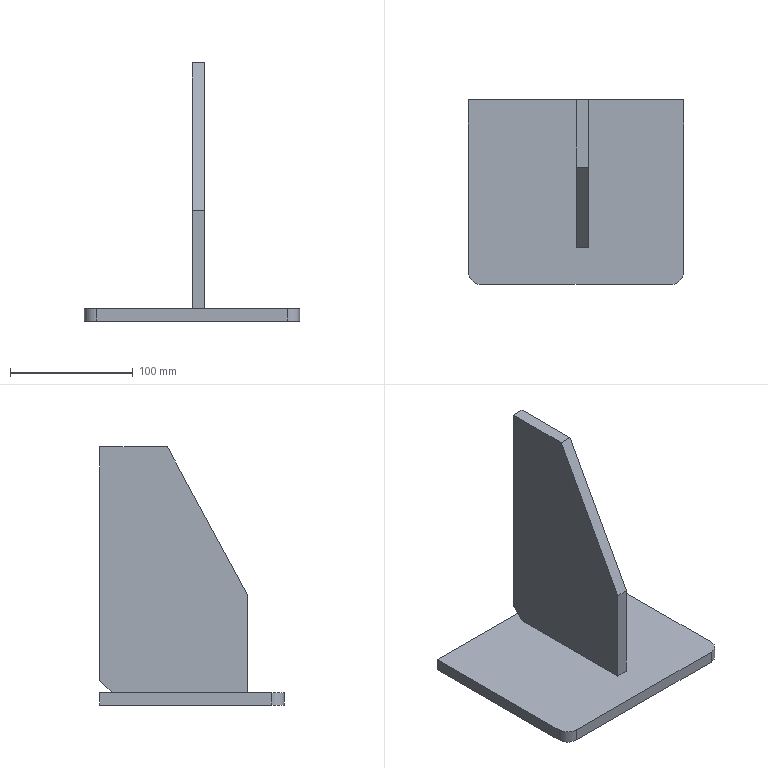Part | STEP file | PN_0029 web-top 10t steel corbel_Default<As Machined> | 2 solids | 16 faces | box 175 x 150 x 209.905 mm | volume 462571 mm3 | plane 13 | cylinder 2 | spline 1 | commonest cylinder face diameters 20 x2
STEP:
#1=CARTESIAN_POINT('',(0.,0.,0.));
#2=DIRECTION('',(0.,0.,1.));
#3=DIRECTION('',(1.,0.,0.));
#4=AXIS2_PLACEMENT_3D('',#1,#2,#3);
#5=CARTESIAN_POINT('',(77.5,-75.,0.));
#6=VERTEX_POINT('',#5);
#7=CARTESIAN_POINT('',(77.5,-75.,10.));
#8=VERTEX_POINT('',#7);
#9=CARTESIAN_POINT('',(77.5,-75.,10.));
#10=DIRECTION('',(0.,0.,1.));
#11=VECTOR('',#10,1.);
#12=LINE('',#9,#11);
#13=CARTESIAN_POINT('',(77.5,-65.,10.));
#14=DIRECTION('',(0.,0.,1.));
#15=DIRECTION('',(1.,0.,0.));
#16=AXIS2_PLACEMENT_3D('',#13,#14,#15);
#17=CYLINDRICAL_SURFACE('',#16,10.);
#18=CARTESIAN_POINT('',(4.712,0.));
#19=DIRECTION('',(0.,1.));
#20=VECTOR('',#19,1.);
#21=LINE('',#18,#20);
#22=(GEOMETRIC_REPRESENTATION_CONTEXT(2)PARAMETRIC_REPRESENTATION_CONTEXT()REPRESENTATION_CONTEXT('',''));
#23=DEFINITIONAL_REPRESENTATION('',(#21),#22);
#24=PCURVE('',#17,#23);
#25=CARTESIAN_POINT('',(-87.5,-75.,10.));
#26=DIRECTION('',(0.,1.,0.));
#27=DIRECTION('',(0.,0.,1.));
#28=AXIS2_PLACEMENT_3D('',#25,#26,#27);
#29=PLANE('',#28);
#30=CARTESIAN_POINT('',(0.,165.));
#31=DIRECTION('',(1.,0.));
#32=VECTOR('',#31,1.);
#33=LINE('',#30,#32);
#34=(GEOMETRIC_REPRESENTATION_CONTEXT(2)PARAMETRIC_REPRESENTATION_CONTEXT()REPRESENTATION_CONTEXT('',''));
#35=DEFINITIONAL_REPRESENTATION('',(#33),#34);
#36=PCURVE('',#29,#35);
#37=SURFACE_CURVE('',#12,(#24,#36),.PCURVE_S1.);
#38=EDGE_CURVE('',#6,#8,#37,.T.);
#39=ORIENTED_EDGE('',*,*,#38,.F.);
#40=CARTESIAN_POINT('',(87.5,-65.,0.));
#41=VERTEX_POINT('',#40);
#42=CARTESIAN_POINT('',(77.5,-65.,0.));
#43=DIRECTION('',(0.,0.,-1.));
#44=DIRECTION('',(1.,0.,0.));
#45=AXIS2_PLACEMENT_3D('',#42,#43,#44);
#46=CIRCLE('',#45,10.);
#47=CARTESIAN_POINT('',(6.283,-10.));
#48=DIRECTION('',(-1.,0.));
#49=VECTOR('',#48,1.);
#50=LINE('',#47,#49);
#51=(GEOMETRIC_REPRESENTATION_CONTEXT(2)PARAMETRIC_REPRESENTATION_CONTEXT()REPRESENTATION_CONTEXT('',''));
#52=DEFINITIONAL_REPRESENTATION('',(#50),#51);
#53=PCURVE('',#17,#52);
#54=CARTESIAN_POINT('',(0.,0.,0.));
#55=DIRECTION('',(0.,0.,1.));
#56=DIRECTION('',(1.,0.,0.));
#57=AXIS2_PLACEMENT_3D('',#54,#55,#56);
#58=PLANE('',#57);
#59=CARTESIAN_POINT('',(87.5,-65.));
#60=CARTESIAN_POINT('',(87.5,-82.321));
#61=CARTESIAN_POINT('',(72.5,-73.66));
#62=CARTESIAN_POINT('',(57.5,-65.));
#63=CARTESIAN_POINT('',(72.5,-56.34));
#64=CARTESIAN_POINT('',(87.5,-47.679));
#65=CARTESIAN_POINT('',(87.5,-65.));
#66=(BOUNDED_CURVE()B_SPLINE_CURVE(2,(#59,#60,#61,#62,#63,#64,#65),.UNSPECIFIED.,.T.,.F.)B_SPLINE_CURVE_WITH_KNOTS((1,2,2,2,2,1),(-2.094,0.,2.094,4.189,6.283,8.378),.UNSPECIFIED.)CURVE()GEOMETRIC_REPRESENTATION_ITEM()RATIONAL_B_SPLINE_CURVE((1.,0.5,1.,0.5,1.,0.5,1.))REPRESENTATION_ITEM(''));
#67=(GEOMETRIC_REPRESENTATION_CONTEXT(2)PARAMETRIC_REPRESENTATION_CONTEXT()REPRESENTATION_CONTEXT('',''));
#68=DEFINITIONAL_REPRESENTATION('',(#66),#67);
#69=PCURVE('',#58,#68);
#70=SURFACE_CURVE('',#46,(#53,#69),.PCURVE_S1.);
#71=EDGE_CURVE('',#41,#6,#70,.T.);
#72=ORIENTED_EDGE('',*,*,#71,.F.);
#73=CARTESIAN_POINT('',(87.5,-65.,10.));
#74=VERTEX_POINT('',#73);
#75=CARTESIAN_POINT('',(87.5,-65.,10.));
#76=DIRECTION('',(0.,0.,-1.));
#77=VECTOR('',#76,1.);
#78=LINE('',#75,#77);
#79=CARTESIAN_POINT('',(6.283,0.));
#80=DIRECTION('',(0.,-1.));
#81=VECTOR('',#80,1.);
#82=LINE('',#79,#81);
#83=(GEOMETRIC_REPRESENTATION_CONTEXT(2)PARAMETRIC_REPRESENTATION_CONTEXT()REPRESENTATION_CONTEXT('',''));
#84=DEFINITIONAL_REPRESENTATION('',(#82),#83);
#85=PCURVE('',#17,#84);
#86=CARTESIAN_POINT('',(87.5,75.,10.));
#87=DIRECTION('',(-1.,0.,0.));
#88=DIRECTION('',(0.,0.,1.));
#89=AXIS2_PLACEMENT_3D('',#86,#87,#88);
#90=PLANE('',#89);
#91=CARTESIAN_POINT('',(0.,-140.));
#92=DIRECTION('',(-1.,0.));
#93=VECTOR('',#92,1.);
#94=LINE('',#91,#93);
#95=(GEOMETRIC_REPRESENTATION_CONTEXT(2)PARAMETRIC_REPRESENTATION_CONTEXT()REPRESENTATION_CONTEXT('',''));
#96=DEFINITIONAL_REPRESENTATION('',(#94),#95);
#97=PCURVE('',#90,#96);
#98=SURFACE_CURVE('',#78,(#85,#97),.PCURVE_S1.);
#99=EDGE_CURVE('',#74,#41,#98,.T.);
#100=ORIENTED_EDGE('',*,*,#99,.F.);
#101=CARTESIAN_POINT('',(77.5,-65.,10.));
#102=DIRECTION('',(0.,0.,1.));
#103=DIRECTION('',(1.,0.,0.));
#104=AXIS2_PLACEMENT_3D('',#101,#102,#103);
#105=CIRCLE('',#104,10.);
#106=CARTESIAN_POINT('',(0.,0.));
#107=DIRECTION('',(1.,0.));
#108=VECTOR('',#107,1.);
#109=LINE('',#106,#108);
#110=(GEOMETRIC_REPRESENTATION_CONTEXT(2)PARAMETRIC_REPRESENTATION_CONTEXT()REPRESENTATION_CONTEXT('',''));
#111=DEFINITIONAL_REPRESENTATION('',(#109),#110);
#112=PCURVE('',#17,#111);
#113=CARTESIAN_POINT('',(0.,0.,10.));
#114=DIRECTION('',(0.,0.,1.));
#115=DIRECTION('',(1.,0.,0.));
#116=AXIS2_PLACEMENT_3D('',#113,#114,#115);
#117=PLANE('',#116);
#118=CARTESIAN_POINT('',(77.5,-65.));
#119=DIRECTION('',(1.,0.));
#120=AXIS2_PLACEMENT_2D('',#118,#119);
#121=CIRCLE('',#120,10.);
#122=(GEOMETRIC_REPRESENTATION_CONTEXT(2)PARAMETRIC_REPRESENTATION_CONTEXT()REPRESENTATION_CONTEXT('',''));
#123=DEFINITIONAL_REPRESENTATION('',(#121),#122);
#124=PCURVE('',#117,#123);
#125=SURFACE_CURVE('',#105,(#112,#124),.PCURVE_S1.);
#126=EDGE_CURVE('',#8,#74,#125,.T.);
#127=ORIENTED_EDGE('',*,*,#126,.F.);
#128=EDGE_LOOP('',(#39,#72,#100,#127));
#129=FACE_BOUND('',#128,.T.);
#130=ADVANCED_FACE('',(#129),#17,.T.);
#131=CARTESIAN_POINT('',(-87.5,-65.,0.));
#132=VERTEX_POINT('',#131);
#133=CARTESIAN_POINT('',(-87.5,-65.,10.));
#134=VERTEX_POINT('',#133);
#135=CARTESIAN_POINT('',(-87.5,-65.,10.));
#136=DIRECTION('',(0.,0.,1.));
#137=VECTOR('',#136,1.);
#138=LINE('',#135,#137);
#139=CARTESIAN_POINT('',(-77.5,-65.,10.));
#140=DIRECTION('',(0.,0.,1.));
#141=DIRECTION('',(1.,0.,0.));
#142=AXIS2_PLACEMENT_3D('',#139,#140,#141);
#143=CYLINDRICAL_SURFACE('',#142,10.);
#144=CARTESIAN_POINT('',(3.142,0.));
#145=DIRECTION('',(0.,1.));
#146=VECTOR('',#145,1.);
#147=LINE('',#144,#146);
#148=(GEOMETRIC_REPRESENTATION_CONTEXT(2)PARAMETRIC_REPRESENTATION_CONTEXT()REPRESENTATION_CONTEXT('',''));
#149=DEFINITIONAL_REPRESENTATION('',(#147),#148);
#150=PCURVE('',#143,#149);
#151=CARTESIAN_POINT('',(-87.5,75.,10.));
#152=DIRECTION('',(1.,0.,0.));
#153=DIRECTION('',(0.,0.,-1.));
#154=AXIS2_PLACEMENT_3D('',#151,#152,#153);
#155=PLANE('',#154);
#156=CARTESIAN_POINT('',(0.,-140.));
#157=DIRECTION('',(-1.,0.));
#158=VECTOR('',#157,1.);
#159=LINE('',#156,#158);
#160=(GEOMETRIC_REPRESENTATION_CONTEXT(2)PARAMETRIC_REPRESENTATION_CONTEXT()REPRESENTATION_CONTEXT('',''));
#161=DEFINITIONAL_REPRESENTATION('',(#159),#160);
#162=PCURVE('',#155,#161);
#163=SURFACE_CURVE('',#138,(#150,#162),.PCURVE_S1.);
#164=EDGE_CURVE('',#132,#134,#163,.T.);
#165=ORIENTED_EDGE('',*,*,#164,.F.);
#166=CARTESIAN_POINT('',(-77.5,-75.,0.));
#167=VERTEX_POINT('',#166);
#168=CARTESIAN_POINT('',(-77.5,-65.,0.));
#169=DIRECTION('',(0.,0.,-1.));
#170=DIRECTION('',(1.,0.,0.));
#171=AXIS2_PLACEMENT_3D('',#168,#169,#170);
#172=CIRCLE('',#171,10.);
#173=CARTESIAN_POINT('',(6.283,-10.));
#174=DIRECTION('',(-1.,0.));
#175=VECTOR('',#174,1.);
#176=LINE('',#173,#175);
#177=(GEOMETRIC_REPRESENTATION_CONTEXT(2)PARAMETRIC_REPRESENTATION_CONTEXT()REPRESENTATION_CONTEXT('',''));
#178=DEFINITIONAL_REPRESENTATION('',(#176),#177);
#179=PCURVE('',#143,#178);
#180=CARTESIAN_POINT('',(-67.5,-65.));
#181=CARTESIAN_POINT('',(-67.5,-82.321));
#182=CARTESIAN_POINT('',(-82.5,-73.66));
#183=CARTESIAN_POINT('',(-97.5,-65.));
#184=CARTESIAN_POINT('',(-82.5,-56.34));
#185=CARTESIAN_POINT('',(-67.5,-47.679));
#186=CARTESIAN_POINT('',(-67.5,-65.));
#187=(BOUNDED_CURVE()B_SPLINE_CURVE(2,(#180,#181,#182,#183,#184,#185,#186),.UNSPECIFIED.,.T.,.F.)B_SPLINE_CURVE_WITH_KNOTS((1,2,2,2,2,1),(-2.094,0.,2.094,4.189,6.283,8.378),.UNSPECIFIED.)CURVE()GEOMETRIC_REPRESENTATION_ITEM()RATIONAL_B_SPLINE_CURVE((1.,0.5,1.,0.5,1.,0.5,1.))REPRESENTATION_ITEM(''));
#188=(GEOMETRIC_REPRESENTATION_CONTEXT(2)PARAMETRIC_REPRESENTATION_CONTEXT()REPRESENTATION_CONTEXT('',''));
#189=DEFINITIONAL_REPRESENTATION('',(#187),#188);
#190=PCURVE('',#58,#189);
#191=SURFACE_CURVE('',#172,(#179,#190),.PCURVE_S1.);
#192=EDGE_CURVE('',#167,#132,#191,.T.);
#193=ORIENTED_EDGE('',*,*,#192,.F.);
#194=CARTESIAN_POINT('',(-77.5,-75.,10.));
#195=VERTEX_POINT('',#194);
#196=CARTESIAN_POINT('',(-77.5,-75.,10.));
#197=DIRECTION('',(0.,0.,-1.));
#198=VECTOR('',#197,1.);
#199=LINE('',#196,#198);
#200=CARTESIAN_POINT('',(4.712,0.));
#201=DIRECTION('',(0.,-1.));
#202=VECTOR('',#201,1.);
#203=LINE('',#200,#202);
#204=(GEOMETRIC_REPRESENTATION_CONTEXT(2)PARAMETRIC_REPRESENTATION_CONTEXT()REPRESENTATION_CONTEXT('',''));
#205=DEFINITIONAL_REPRESENTATION('',(#203),#204);
#206=PCURVE('',#143,#205);
#207=CARTESIAN_POINT('',(0.,10.));
#208=DIRECTION('',(-1.,0.));
#209=VECTOR('',#208,1.);
#210=LINE('',#207,#209);
#211=(GEOMETRIC_REPRESENTATION_CONTEXT(2)PARAMETRIC_REPRESENTATION_CONTEXT()REPRESENTATION_CONTEXT('',''));
#212=DEFINITIONAL_REPRESENTATION('',(#210),#211);
#213=PCURVE('',#29,#212);
#214=SURFACE_CURVE('',#199,(#206,#213),.PCURVE_S1.);
#215=EDGE_CURVE('',#195,#167,#214,.T.);
#216=ORIENTED_EDGE('',*,*,#215,.F.);
#217=CARTESIAN_POINT('',(-77.5,-65.,10.));
#218=DIRECTION('',(0.,0.,1.));
#219=DIRECTION('',(1.,0.,0.));
#220=AXIS2_PLACEMENT_3D('',#217,#218,#219);
#221=CIRCLE('',#220,10.);
#222=CARTESIAN_POINT('',(0.,0.));
#223=DIRECTION('',(1.,0.));
#224=VECTOR('',#223,1.);
#225=LINE('',#222,#224);
#226=(GEOMETRIC_REPRESENTATION_CONTEXT(2)PARAMETRIC_REPRESENTATION_CONTEXT()REPRESENTATION_CONTEXT('',''));
#227=DEFINITIONAL_REPRESENTATION('',(#225),#226);
#228=PCURVE('',#143,#227);
#229=CARTESIAN_POINT('',(-77.5,-65.));
#230=DIRECTION('',(1.,0.));
#231=AXIS2_PLACEMENT_2D('',#229,#230);
#232=CIRCLE('',#231,10.);
#233=(GEOMETRIC_REPRESENTATION_CONTEXT(2)PARAMETRIC_REPRESENTATION_CONTEXT()REPRESENTATION_CONTEXT('',''));
#234=DEFINITIONAL_REPRESENTATION('',(#232),#233);
#235=PCURVE('',#117,#234);
#236=SURFACE_CURVE('',#221,(#228,#235),.PCURVE_S1.);
#237=EDGE_CURVE('',#134,#195,#236,.T.);
#238=ORIENTED_EDGE('',*,*,#237,.F.);
#239=EDGE_LOOP('',(#165,#193,#216,#238));
#240=FACE_BOUND('',#239,.T.);
#241=ADVANCED_FACE('',(#240),#143,.T.);
#242=CARTESIAN_POINT('',(87.5,75.,10.));
#243=VERTEX_POINT('',#242);
#244=CARTESIAN_POINT('',(87.5,75.,10.));
#245=DIRECTION('',(0.,1.,0.));
#246=VECTOR('',#245,1.);
#247=LINE('',#244,#246);
#248=CARTESIAN_POINT('',(0.,0.));
#249=DIRECTION('',(0.,1.));
#250=VECTOR('',#249,1.);
#251=LINE('',#248,#250);
#252=(GEOMETRIC_REPRESENTATION_CONTEXT(2)PARAMETRIC_REPRESENTATION_CONTEXT()REPRESENTATION_CONTEXT('',''));
#253=DEFINITIONAL_REPRESENTATION('',(#251),#252);
#254=PCURVE('',#90,#253);
#255=CARTESIAN_POINT('',(87.5,75.));
#256=DIRECTION('',(0.,1.));
#257=VECTOR('',#256,1.);
#258=LINE('',#255,#257);
#259=(GEOMETRIC_REPRESENTATION_CONTEXT(2)PARAMETRIC_REPRESENTATION_CONTEXT()REPRESENTATION_CONTEXT('',''));
#260=DEFINITIONAL_REPRESENTATION('',(#258),#259);
#261=PCURVE('',#117,#260);
#262=SURFACE_CURVE('',#247,(#254,#261),.PCURVE_S1.);
#263=EDGE_CURVE('',#74,#243,#262,.T.);
#264=ORIENTED_EDGE('',*,*,#263,.F.);
#265=ORIENTED_EDGE('',*,*,#99,.T.);
#266=CARTESIAN_POINT('',(87.5,75.,0.));
#267=VERTEX_POINT('',#266);
#268=CARTESIAN_POINT('',(87.5,75.,0.));
#269=DIRECTION('',(0.,1.,0.));
#270=VECTOR('',#269,1.);
#271=LINE('',#268,#270);
#272=CARTESIAN_POINT('',(-10.,0.));
#273=DIRECTION('',(0.,1.));
#274=VECTOR('',#273,1.);
#275=LINE('',#272,#274);
#276=(GEOMETRIC_REPRESENTATION_CONTEXT(2)PARAMETRIC_REPRESENTATION_CONTEXT()REPRESENTATION_CONTEXT('',''));
#277=DEFINITIONAL_REPRESENTATION('',(#275),#276);
#278=PCURVE('',#90,#277);
#279=CARTESIAN_POINT('',(87.5,75.));
#280=DIRECTION('',(0.,1.));
#281=VECTOR('',#280,1.);
#282=LINE('',#279,#281);
#283=(GEOMETRIC_REPRESENTATION_CONTEXT(2)PARAMETRIC_REPRESENTATION_CONTEXT()REPRESENTATION_CONTEXT('',''));
#284=DEFINITIONAL_REPRESENTATION('',(#282),#283);
#285=PCURVE('',#58,#284);
#286=SURFACE_CURVE('',#271,(#278,#285),.PCURVE_S1.);
#287=EDGE_CURVE('',#41,#267,#286,.T.);
#288=ORIENTED_EDGE('',*,*,#287,.T.);
#289=CARTESIAN_POINT('',(87.5,75.,10.));
#290=DIRECTION('',(0.,0.,-1.));
#291=VECTOR('',#290,1.);
#292=LINE('',#289,#291);
#293=CARTESIAN_POINT('',(0.,0.));
#294=DIRECTION('',(-1.,0.));
#295=VECTOR('',#294,1.);
#296=LINE('',#293,#295);
#297=(GEOMETRIC_REPRESENTATION_CONTEXT(2)PARAMETRIC_REPRESENTATION_CONTEXT()REPRESENTATION_CONTEXT('',''));
#298=DEFINITIONAL_REPRESENTATION('',(#296),#297);
#299=PCURVE('',#90,#298);
#300=CARTESIAN_POINT('',(-87.5,75.,10.));
#301=DIRECTION('',(0.,-1.,0.));
#302=DIRECTION('',(0.,0.,-1.));
#303=AXIS2_PLACEMENT_3D('',#300,#301,#302);
#304=PLANE('',#303);
#305=CARTESIAN_POINT('',(0.,175.));
#306=DIRECTION('',(1.,0.));
#307=VECTOR('',#306,1.);
#308=LINE('',#305,#307);
#309=(GEOMETRIC_REPRESENTATION_CONTEXT(2)PARAMETRIC_REPRESENTATION_CONTEXT()REPRESENTATION_CONTEXT('',''));
#310=DEFINITIONAL_REPRESENTATION('',(#308),#309);
#311=PCURVE('',#304,#310);
#312=SURFACE_CURVE('',#292,(#299,#311),.PCURVE_S1.);
#313=EDGE_CURVE('',#243,#267,#312,.T.);
#314=ORIENTED_EDGE('',*,*,#313,.F.);
#315=EDGE_LOOP('',(#264,#265,#288,#314));
#316=FACE_BOUND('',#315,.T.);
#317=ADVANCED_FACE('',(#316),#90,.F.);
#318=CARTESIAN_POINT('',(-87.5,75.,0.));
#319=VERTEX_POINT('',#318);
#320=CARTESIAN_POINT('',(-87.5,75.,0.));
#321=DIRECTION('',(-1.,0.,0.));
#322=VECTOR('',#321,1.);
#323=LINE('',#320,#322);
#324=CARTESIAN_POINT('',(10.,0.));
#325=DIRECTION('',(0.,-1.));
#326=VECTOR('',#325,1.);
#327=LINE('',#324,#326);
#328=(GEOMETRIC_REPRESENTATION_CONTEXT(2)PARAMETRIC_REPRESENTATION_CONTEXT()REPRESENTATION_CONTEXT('',''));
#329=DEFINITIONAL_REPRESENTATION('',(#327),#328);
#330=PCURVE('',#304,#329);
#331=CARTESIAN_POINT('',(-87.5,75.));
#332=DIRECTION('',(-1.,0.));
#333=VECTOR('',#332,1.);
#334=LINE('',#331,#333);
#335=(GEOMETRIC_REPRESENTATION_CONTEXT(2)PARAMETRIC_REPRESENTATION_CONTEXT()REPRESENTATION_CONTEXT('',''));
#336=DEFINITIONAL_REPRESENTATION('',(#334),#335);
#337=PCURVE('',#58,#336);
#338=SURFACE_CURVE('',#323,(#330,#337),.PCURVE_S1.);
#339=EDGE_CURVE('',#267,#319,#338,.T.);
#340=ORIENTED_EDGE('',*,*,#339,.T.);
#341=CARTESIAN_POINT('',(-87.5,75.,10.));
#342=VERTEX_POINT('',#341);
#343=CARTESIAN_POINT('',(-87.5,75.,10.));
#344=DIRECTION('',(0.,0.,-1.));
#345=VECTOR('',#344,1.);
#346=LINE('',#343,#345);
#347=CARTESIAN_POINT('',(0.,0.));
#348=DIRECTION('',(1.,0.));
#349=VECTOR('',#348,1.);
#350=LINE('',#347,#349);
#351=(GEOMETRIC_REPRESENTATION_CONTEXT(2)PARAMETRIC_REPRESENTATION_CONTEXT()REPRESENTATION_CONTEXT('',''));
#352=DEFINITIONAL_REPRESENTATION('',(#350),#351);
#353=PCURVE('',#304,#352);
#354=CARTESIAN_POINT('',(0.,0.));
#355=DIRECTION('',(1.,0.));
#356=VECTOR('',#355,1.);
#357=LINE('',#354,#356);
#358=(GEOMETRIC_REPRESENTATION_CONTEXT(2)PARAMETRIC_REPRESENTATION_CONTEXT()REPRESENTATION_CONTEXT('',''));
#359=DEFINITIONAL_REPRESENTATION('',(#357),#358);
#360=PCURVE('',#155,#359);
#361=SURFACE_CURVE('',#346,(#353,#360),.PCURVE_S1.);
#362=EDGE_CURVE('',#342,#319,#361,.T.);
#363=ORIENTED_EDGE('',*,*,#362,.F.);
#364=CARTESIAN_POINT('',(-87.5,75.,10.));
#365=DIRECTION('',(-1.,0.,0.));
#366=VECTOR('',#365,1.);
#367=LINE('',#364,#366);
#368=CARTESIAN_POINT('',(0.,0.));
#369=DIRECTION('',(0.,-1.));
#370=VECTOR('',#369,1.);
#371=LINE('',#368,#370);
#372=(GEOMETRIC_REPRESENTATION_CONTEXT(2)PARAMETRIC_REPRESENTATION_CONTEXT()REPRESENTATION_CONTEXT('',''));
#373=DEFINITIONAL_REPRESENTATION('',(#371),#372);
#374=PCURVE('',#304,#373);
#375=CARTESIAN_POINT('',(-87.5,75.));
#376=DIRECTION('',(-1.,0.));
#377=VECTOR('',#376,1.);
#378=LINE('',#375,#377);
#379=(GEOMETRIC_REPRESENTATION_CONTEXT(2)PARAMETRIC_REPRESENTATION_CONTEXT()REPRESENTATION_CONTEXT('',''));
#380=DEFINITIONAL_REPRESENTATION('',(#378),#379);
#381=PCURVE('',#117,#380);
#382=SURFACE_CURVE('',#367,(#374,#381),.PCURVE_S1.);
#383=EDGE_CURVE('',#243,#342,#382,.T.);
#384=ORIENTED_EDGE('',*,*,#383,.F.);
#385=ORIENTED_EDGE('',*,*,#313,.T.);
#386=EDGE_LOOP('',(#340,#363,#384,#385));
#387=FACE_BOUND('',#386,.T.);
#388=ADVANCED_FACE('',(#387),#304,.F.);
#389=CARTESIAN_POINT('',(-87.5,75.,0.));
#390=DIRECTION('',(0.,-1.,0.));
#391=VECTOR('',#390,1.);
#392=LINE('',#389,#391);
#393=CARTESIAN_POINT('',(10.,0.));
#394=DIRECTION('',(0.,-1.));
#395=VECTOR('',#394,1.);
#396=LINE('',#393,#395);
#397=(GEOMETRIC_REPRESENTATION_CONTEXT(2)PARAMETRIC_REPRESENTATION_CONTEXT()REPRESENTATION_CONTEXT('',''));
#398=DEFINITIONAL_REPRESENTATION('',(#396),#397);
#399=PCURVE('',#155,#398);
#400=CARTESIAN_POINT('',(-87.5,75.));
#401=DIRECTION('',(0.,-1.));
#402=VECTOR('',#401,1.);
#403=LINE('',#400,#402);
#404=(GEOMETRIC_REPRESENTATION_CONTEXT(2)PARAMETRIC_REPRESENTATION_CONTEXT()REPRESENTATION_CONTEXT('',''));
#405=DEFINITIONAL_REPRESENTATION('',(#403),#404);
#406=PCURVE('',#58,#405);
#407=SURFACE_CURVE('',#392,(#399,#406),.PCURVE_S1.);
#408=EDGE_CURVE('',#319,#132,#407,.T.);
#409=ORIENTED_EDGE('',*,*,#408,.T.);
#410=ORIENTED_EDGE('',*,*,#164,.T.);
#411=CARTESIAN_POINT('',(-87.5,75.,10.));
#412=DIRECTION('',(0.,-1.,0.));
#413=VECTOR('',#412,1.);
#414=LINE('',#411,#413);
#415=CARTESIAN_POINT('',(0.,0.));
#416=DIRECTION('',(0.,-1.));
#417=VECTOR('',#416,1.);
#418=LINE('',#415,#417);
#419=(GEOMETRIC_REPRESENTATION_CONTEXT(2)PARAMETRIC_REPRESENTATION_CONTEXT()REPRESENTATION_CONTEXT('',''));
#420=DEFINITIONAL_REPRESENTATION('',(#418),#419);
#421=PCURVE('',#155,#420);
#422=CARTESIAN_POINT('',(-87.5,75.));
#423=DIRECTION('',(0.,-1.));
#424=VECTOR('',#423,1.);
#425=LINE('',#422,#424);
#426=(GEOMETRIC_REPRESENTATION_CONTEXT(2)PARAMETRIC_REPRESENTATION_CONTEXT()REPRESENTATION_CONTEXT('',''));
#427=DEFINITIONAL_REPRESENTATION('',(#425),#426);
#428=PCURVE('',#117,#427);
#429=SURFACE_CURVE('',#414,(#421,#428),.PCURVE_S1.);
#430=EDGE_CURVE('',#342,#134,#429,.T.);
#431=ORIENTED_EDGE('',*,*,#430,.F.);
#432=ORIENTED_EDGE('',*,*,#362,.T.);
#433=EDGE_LOOP('',(#409,#410,#431,#432));
#434=FACE_BOUND('',#433,.T.);
#435=ADVANCED_FACE('',(#434),#155,.F.);
#436=CARTESIAN_POINT('',(-87.5,-75.,0.));
#437=DIRECTION('',(1.,0.,0.));
#438=VECTOR('',#437,1.);
#439=LINE('',#436,#438);
#440=CARTESIAN_POINT('',(-10.,0.));
#441=DIRECTION('',(0.,1.));
#442=VECTOR('',#441,1.);
#443=LINE('',#440,#442);
#444=(GEOMETRIC_REPRESENTATION_CONTEXT(2)PARAMETRIC_REPRESENTATION_CONTEXT()REPRESENTATION_CONTEXT('',''));
#445=DEFINITIONAL_REPRESENTATION('',(#443),#444);
#446=PCURVE('',#29,#445);
#447=CARTESIAN_POINT('',(-87.5,-75.));
#448=DIRECTION('',(1.,0.));
#449=VECTOR('',#448,1.);
#450=LINE('',#447,#449);
#451=(GEOMETRIC_REPRESENTATION_CONTEXT(2)PARAMETRIC_REPRESENTATION_CONTEXT()REPRESENTATION_CONTEXT('',''));
#452=DEFINITIONAL_REPRESENTATION('',(#450),#451);
#453=PCURVE('',#58,#452);
#454=SURFACE_CURVE('',#439,(#446,#453),.PCURVE_S1.);
#455=EDGE_CURVE('',#167,#6,#454,.T.);
#456=ORIENTED_EDGE('',*,*,#455,.T.);
#457=ORIENTED_EDGE('',*,*,#38,.T.);
#458=CARTESIAN_POINT('',(-87.5,-75.,10.));
#459=DIRECTION('',(1.,0.,0.));
#460=VECTOR('',#459,1.);
#461=LINE('',#458,#460);
#462=CARTESIAN_POINT('',(0.,0.));
#463=DIRECTION('',(0.,1.));
#464=VECTOR('',#463,1.);
#465=LINE('',#462,#464);
#466=(GEOMETRIC_REPRESENTATION_CONTEXT(2)PARAMETRIC_REPRESENTATION_CONTEXT()REPRESENTATION_CONTEXT('',''));
#467=DEFINITIONAL_REPRESENTATION('',(#465),#466);
#468=PCURVE('',#29,#467);
#469=CARTESIAN_POINT('',(-87.5,-75.));
#470=DIRECTION('',(1.,0.));
#471=VECTOR('',#470,1.);
#472=LINE('',#469,#471);
#473=(GEOMETRIC_REPRESENTATION_CONTEXT(2)PARAMETRIC_REPRESENTATION_CONTEXT()REPRESENTATION_CONTEXT('',''));
#474=DEFINITIONAL_REPRESENTATION('',(#472),#473);
#475=PCURVE('',#117,#474);
#476=SURFACE_CURVE('',#461,(#468,#475),.PCURVE_S1.);
#477=EDGE_CURVE('',#195,#8,#476,.T.);
#478=ORIENTED_EDGE('',*,*,#477,.F.);
#479=ORIENTED_EDGE('',*,*,#215,.T.);
#480=EDGE_LOOP('',(#456,#457,#478,#479));
#481=FACE_BOUND('',#480,.T.);
#482=ADVANCED_FACE('',(#481),#29,.F.);
#483=ORIENTED_EDGE('',*,*,#477,.T.);
#484=ORIENTED_EDGE('',*,*,#126,.T.);
#485=ORIENTED_EDGE('',*,*,#263,.T.);
#486=ORIENTED_EDGE('',*,*,#383,.T.);
#487=ORIENTED_EDGE('',*,*,#430,.T.);
#488=ORIENTED_EDGE('',*,*,#237,.T.);
#489=EDGE_LOOP('',(#483,#484,#485,#486,#487,#488));
#490=FACE_BOUND('',#489,.T.);
#491=ADVANCED_FACE('',(#490),#117,.T.);
#492=ORIENTED_EDGE('',*,*,#287,.F.);
#493=ORIENTED_EDGE('',*,*,#71,.T.);
#494=ORIENTED_EDGE('',*,*,#455,.F.);
#495=ORIENTED_EDGE('',*,*,#192,.T.);
#496=ORIENTED_EDGE('',*,*,#408,.F.);
#497=ORIENTED_EDGE('',*,*,#339,.F.);
#498=EDGE_LOOP('',(#492,#493,#494,#495,#496,#497));
#499=FACE_BOUND('',#498,.T.);
#500=ADVANCED_FACE('',(#499),#58,.F.);
#501=CLOSED_SHELL('',(#130,#241,#317,#388,#435,#482,#491,#500));
#502=MANIFOLD_SOLID_BREP('',#501);
#503=CARTESIAN_POINT('',(0.,64.998,9.905));
#504=VERTEX_POINT('',#503);
#505=CARTESIAN_POINT('',(10.,64.998,9.905));
#506=VERTEX_POINT('',#505);
#507=CARTESIAN_POINT('',(10.,64.998,9.905));
#508=DIRECTION('',(1.,0.,0.));
#509=VECTOR('',#508,1.);
#510=LINE('',#507,#509);
#511=CARTESIAN_POINT('',(10.,64.998,9.905));
#512=DIRECTION('',(0.,-0.7071,0.7071));
#513=DIRECTION('',(1.,0.,0.));
#514=AXIS2_PLACEMENT_3D('',#511,#512,#513);
#515=PLANE('',#514);
#516=CARTESIAN_POINT('',(0.,0.));
#517=DIRECTION('',(1.,0.));
#518=VECTOR('',#517,1.);
#519=LINE('',#516,#518);
#520=(GEOMETRIC_REPRESENTATION_CONTEXT(2)PARAMETRIC_REPRESENTATION_CONTEXT()REPRESENTATION_CONTEXT('',''));
#521=DEFINITIONAL_REPRESENTATION('',(#519),#520);
#522=PCURVE('',#515,#521);
#523=CARTESIAN_POINT('',(10.,74.998,9.905));
#524=DIRECTION('',(0.,0.,1.));
#525=DIRECTION('',(1.,0.,0.));
#526=AXIS2_PLACEMENT_3D('',#523,#524,#525);
#527=PLANE('',#526);
#528=CARTESIAN_POINT('',(0.,-10.));
#529=DIRECTION('',(1.,0.));
#530=VECTOR('',#529,1.);
#531=LINE('',#528,#530);
#532=(GEOMETRIC_REPRESENTATION_CONTEXT(2)PARAMETRIC_REPRESENTATION_CONTEXT()REPRESENTATION_CONTEXT('',''));
#533=DEFINITIONAL_REPRESENTATION('',(#531),#532);
#534=PCURVE('',#527,#533);
#535=SURFACE_CURVE('',#510,(#522,#534),.PCURVE_S1.);
#536=EDGE_CURVE('',#504,#506,#535,.T.);
#537=ORIENTED_EDGE('',*,*,#536,.F.);
#538=CARTESIAN_POINT('',(0.,74.998,19.905));
#539=VERTEX_POINT('',#538);
#540=CARTESIAN_POINT('',(0.,-1.144,-56.236));
#541=DIRECTION('',(0.,-0.7071,-0.7071));
#542=VECTOR('',#541,1.);
#543=LINE('',#540,#542);
#544=CARTESIAN_POINT('',(-10.,-93.538));
#545=DIRECTION('',(0.,-1.));
#546=VECTOR('',#545,1.);
#547=LINE('',#544,#546);
#548=(GEOMETRIC_REPRESENTATION_CONTEXT(2)PARAMETRIC_REPRESENTATION_CONTEXT()REPRESENTATION_CONTEXT('',''));
#549=DEFINITIONAL_REPRESENTATION('',(#547),#548);
#550=PCURVE('',#515,#549);
#551=CARTESIAN_POINT('',(0.,-37.84,-19.54));
#552=DIRECTION('',(-1.,0.,0.));
#553=DIRECTION('',(0.,0.,1.));
#554=AXIS2_PLACEMENT_3D('',#551,#552,#553);
#555=PLANE('',#554);
#556=CARTESIAN_POINT('',(-36.696,36.696));
#557=DIRECTION('',(-0.7071,-0.7071));
#558=VECTOR('',#557,1.);
#559=LINE('',#556,#558);
#560=(GEOMETRIC_REPRESENTATION_CONTEXT(2)PARAMETRIC_REPRESENTATION_CONTEXT()REPRESENTATION_CONTEXT('',''));
#561=DEFINITIONAL_REPRESENTATION('',(#559),#560);
#562=PCURVE('',#555,#561);
#563=SURFACE_CURVE('',#543,(#550,#562),.PCURVE_S1.);
#564=EDGE_CURVE('',#539,#504,#563,.T.);
#565=ORIENTED_EDGE('',*,*,#564,.F.);
#566=CARTESIAN_POINT('',(10.,74.998,19.905));
#567=VERTEX_POINT('',#566);
#568=CARTESIAN_POINT('',(10.,74.998,19.905));
#569=DIRECTION('',(-1.,0.,0.));
#570=VECTOR('',#569,1.);
#571=LINE('',#568,#570);
#572=CARTESIAN_POINT('',(0.,14.142));
#573=DIRECTION('',(-1.,0.));
#574=VECTOR('',#573,1.);
#575=LINE('',#572,#574);
#576=(GEOMETRIC_REPRESENTATION_CONTEXT(2)PARAMETRIC_REPRESENTATION_CONTEXT()REPRESENTATION_CONTEXT('',''));
#577=DEFINITIONAL_REPRESENTATION('',(#575),#576);
#578=PCURVE('',#515,#577);
#579=CARTESIAN_POINT('',(10.,74.998,9.905));
#580=DIRECTION('',(0.,-1.,0.));
#581=DIRECTION('',(0.,0.,-1.));
#582=AXIS2_PLACEMENT_3D('',#579,#580,#581);
#583=PLANE('',#582);
#584=CARTESIAN_POINT('',(-10.,0.));
#585=DIRECTION('',(0.,-1.));
#586=VECTOR('',#585,1.);
#587=LINE('',#584,#586);
#588=(GEOMETRIC_REPRESENTATION_CONTEXT(2)PARAMETRIC_REPRESENTATION_CONTEXT()REPRESENTATION_CONTEXT('',''));
#589=DEFINITIONAL_REPRESENTATION('',(#587),#588);
#590=PCURVE('',#583,#589);
#591=SURFACE_CURVE('',#571,(#578,#590),.PCURVE_S1.);
#592=EDGE_CURVE('',#567,#539,#591,.T.);
#593=ORIENTED_EDGE('',*,*,#592,.F.);
#594=CARTESIAN_POINT('',(10.,64.998,9.905));
#595=DIRECTION('',(0.,0.7071,0.7071));
#596=VECTOR('',#595,1.);
#597=LINE('',#594,#596);
#598=CARTESIAN_POINT('',(0.,0.));
#599=DIRECTION('',(0.,1.));
#600=VECTOR('',#599,1.);
#601=LINE('',#598,#600);
#602=(GEOMETRIC_REPRESENTATION_CONTEXT(2)PARAMETRIC_REPRESENTATION_CONTEXT()REPRESENTATION_CONTEXT('',''));
#603=DEFINITIONAL_REPRESENTATION('',(#601),#602);
#604=PCURVE('',#515,#603);
#605=CARTESIAN_POINT('',(10.,-37.84,-19.54));
#606=DIRECTION('',(-1.,0.,0.));
#607=DIRECTION('',(0.,0.,1.));
#608=AXIS2_PLACEMENT_3D('',#605,#606,#607);
#609=PLANE('',#608);
#610=CARTESIAN_POINT('',(29.445,102.838));
#611=DIRECTION('',(0.7071,0.7071));
#612=VECTOR('',#611,1.);
#613=LINE('',#610,#612);
#614=(GEOMETRIC_REPRESENTATION_CONTEXT(2)PARAMETRIC_REPRESENTATION_CONTEXT()REPRESENTATION_CONTEXT('',''));
#615=DEFINITIONAL_REPRESENTATION('',(#613),#614);
#616=PCURVE('',#609,#615);
#617=SURFACE_CURVE('',#597,(#604,#616),.PCURVE_S1.);
#618=EDGE_CURVE('',#506,#567,#617,.T.);
#619=ORIENTED_EDGE('',*,*,#618,.F.);
#620=EDGE_LOOP('',(#537,#565,#593,#619));
#621=FACE_BOUND('',#620,.T.);
#622=ADVANCED_FACE('',(#621),#515,.F.);
#623=CARTESIAN_POINT('',(0.,19.998,209.905));
#624=VERTEX_POINT('',#623);
#625=CARTESIAN_POINT('',(10.,19.998,209.905));
#626=VERTEX_POINT('',#625);
#627=CARTESIAN_POINT('',(0.,19.998,209.905));
#628=CARTESIAN_POINT('',(3.333,19.998,209.905));
#629=CARTESIAN_POINT('',(6.667,19.998,209.905));
#630=CARTESIAN_POINT('',(10.,19.998,209.905));
#631=B_SPLINE_CURVE_WITH_KNOTS('',3,(#627,#628,#629,#630),.UNSPECIFIED.,.F.,.F.,(4,4),(0.,1.),.PIECEWISE_BEZIER_KNOTS.);
#632=CARTESIAN_POINT('',(-1.,19.998,209.905));
#633=CARTESIAN_POINT('',(3.,19.998,209.905));
#634=CARTESIAN_POINT('',(7.,19.998,209.905));
#635=CARTESIAN_POINT('',(11.,19.998,209.905));
#636=CARTESIAN_POINT('',(-1.,-45.002,89.905));
#637=CARTESIAN_POINT('',(3.,-45.002,89.905));
#638=CARTESIAN_POINT('',(7.,-45.002,89.905));
#639=CARTESIAN_POINT('',(11.,-45.002,89.905));
#640=B_SPLINE_SURFACE_WITH_KNOTS('',1,3,((#632,#633,#634,#635),(#636,#637,#638,#639)),.UNSPECIFIED.,.F.,.F.,.F.,(2,2),(4,4),(0.,1.),(-0.011,0.001),.PIECEWISE_BEZIER_KNOTS.);
#641=CARTESIAN_POINT('',(0.,-0.01));
#642=CARTESIAN_POINT('',(0.,0.));
#643=B_SPLINE_CURVE_WITH_KNOTS('',1,(#641,#642),.UNSPECIFIED.,.F.,.F.,(2,2),(0.,1.),.PIECEWISE_BEZIER_KNOTS.);
#644=(GEOMETRIC_REPRESENTATION_CONTEXT(2)PARAMETRIC_REPRESENTATION_CONTEXT()REPRESENTATION_CONTEXT('',''));
#645=DEFINITIONAL_REPRESENTATION('',(#643),#644);
#646=PCURVE('',#640,#645);
#647=CARTESIAN_POINT('',(10.,74.998,209.905));
#648=DIRECTION('',(0.,0.,-1.));
#649=DIRECTION('',(-1.,0.,0.));
#650=AXIS2_PLACEMENT_3D('',#647,#648,#649);
#651=PLANE('',#650);
#652=CARTESIAN_POINT('',(10.,-55.));
#653=CARTESIAN_POINT('',(6.667,-55.));
#654=CARTESIAN_POINT('',(3.333,-55.));
#655=CARTESIAN_POINT('',(0.,-55.));
#656=B_SPLINE_CURVE_WITH_KNOTS('',3,(#652,#653,#654,#655),.UNSPECIFIED.,.F.,.F.,(4,4),(0.,1.),.PIECEWISE_BEZIER_KNOTS.);
#657=(GEOMETRIC_REPRESENTATION_CONTEXT(2)PARAMETRIC_REPRESENTATION_CONTEXT()REPRESENTATION_CONTEXT('',''));
#658=DEFINITIONAL_REPRESENTATION('',(#656),#657);
#659=PCURVE('',#651,#658);
#660=SURFACE_CURVE('',#631,(#646,#659),.PCURVE_S1.);
#661=EDGE_CURVE('',#624,#626,#660,.T.);
#662=ORIENTED_EDGE('',*,*,#661,.F.);
#663=CARTESIAN_POINT('',(0.,-45.002,89.905));
#664=VERTEX_POINT('',#663);
#665=CARTESIAN_POINT('',(0.,-45.002,89.905));
#666=CARTESIAN_POINT('',(0.,-23.336,129.905));
#667=CARTESIAN_POINT('',(0.,-1.669,169.905));
#668=CARTESIAN_POINT('',(0.,19.998,209.905));
#669=B_SPLINE_CURVE_WITH_KNOTS('',3,(#665,#666,#667,#668),.UNSPECIFIED.,.F.,.F.,(4,4),(0.,1.),.PIECEWISE_BEZIER_KNOTS.);
#670=CARTESIAN_POINT('',(1.,-0.01));
#671=DIRECTION('',(-1.,0.));
#672=VECTOR('',#671,1.);
#673=LINE('',#670,#672);
#674=(GEOMETRIC_REPRESENTATION_CONTEXT(2)PARAMETRIC_REPRESENTATION_CONTEXT()REPRESENTATION_CONTEXT('',''));
#675=DEFINITIONAL_REPRESENTATION('',(#673),#674);
#676=PCURVE('',#640,#675);
#677=CARTESIAN_POINT('',(109.445,-7.162));
#678=CARTESIAN_POINT('',(149.445,14.504));
#679=CARTESIAN_POINT('',(189.445,36.171));
#680=CARTESIAN_POINT('',(229.445,57.838));
#681=B_SPLINE_CURVE_WITH_KNOTS('',3,(#677,#678,#679,#680),.UNSPECIFIED.,.F.,.F.,(4,4),(0.,1.),.PIECEWISE_BEZIER_KNOTS.);
#682=(GEOMETRIC_REPRESENTATION_CONTEXT(2)PARAMETRIC_REPRESENTATION_CONTEXT()REPRESENTATION_CONTEXT('',''));
#683=DEFINITIONAL_REPRESENTATION('',(#681),#682);
#684=PCURVE('',#555,#683);
#685=SURFACE_CURVE('',#669,(#676,#684),.PCURVE_S1.);
#686=EDGE_CURVE('',#664,#624,#685,.T.);
#687=ORIENTED_EDGE('',*,*,#686,.F.);
#688=CARTESIAN_POINT('',(10.,-45.002,89.905));
#689=VERTEX_POINT('',#688);
#690=CARTESIAN_POINT('',(10.,-45.002,89.905));
#691=CARTESIAN_POINT('',(6.667,-45.002,89.905));
#692=CARTESIAN_POINT('',(3.333,-45.002,89.905));
#693=CARTESIAN_POINT('',(0.,-45.002,89.905));
#694=B_SPLINE_CURVE_WITH_KNOTS('',3,(#690,#691,#692,#693),.UNSPECIFIED.,.F.,.F.,(4,4),(0.,1.),.PIECEWISE_BEZIER_KNOTS.);
#695=CARTESIAN_POINT('',(1.,0.));
#696=CARTESIAN_POINT('',(1.,-0.01));
#697=B_SPLINE_CURVE_WITH_KNOTS('',1,(#695,#696),.UNSPECIFIED.,.F.,.F.,(2,2),(0.,1.),.PIECEWISE_BEZIER_KNOTS.);
#698=(GEOMETRIC_REPRESENTATION_CONTEXT(2)PARAMETRIC_REPRESENTATION_CONTEXT()REPRESENTATION_CONTEXT('',''));
#699=DEFINITIONAL_REPRESENTATION('',(#697),#698);
#700=PCURVE('',#640,#699);
#701=CARTESIAN_POINT('',(10.,-45.002,9.905));
#702=DIRECTION('',(0.,1.,0.));
#703=DIRECTION('',(0.,0.,1.));
#704=AXIS2_PLACEMENT_3D('',#701,#702,#703);
#705=PLANE('',#704);
#706=CARTESIAN_POINT('',(80.,0.));
#707=CARTESIAN_POINT('',(80.,-3.333));
#708=CARTESIAN_POINT('',(80.,-6.667));
#709=CARTESIAN_POINT('',(80.,-10.));
#710=B_SPLINE_CURVE_WITH_KNOTS('',3,(#706,#707,#708,#709),.UNSPECIFIED.,.F.,.F.,(4,4),(0.,1.),.PIECEWISE_BEZIER_KNOTS.);
#711=(GEOMETRIC_REPRESENTATION_CONTEXT(2)PARAMETRIC_REPRESENTATION_CONTEXT()REPRESENTATION_CONTEXT('',''));
#712=DEFINITIONAL_REPRESENTATION('',(#710),#711);
#713=PCURVE('',#705,#712);
#714=SURFACE_CURVE('',#694,(#700,#713),.PCURVE_S1.);
#715=EDGE_CURVE('',#689,#664,#714,.T.);
#716=ORIENTED_EDGE('',*,*,#715,.F.);
#717=CARTESIAN_POINT('',(10.,19.998,209.905));
#718=CARTESIAN_POINT('',(10.,-1.669,169.905));
#719=CARTESIAN_POINT('',(10.,-23.336,129.905));
#720=CARTESIAN_POINT('',(10.,-45.002,89.905));
#721=B_SPLINE_CURVE_WITH_KNOTS('',3,(#717,#718,#719,#720),.UNSPECIFIED.,.F.,.F.,(4,4),(0.,1.),.PIECEWISE_BEZIER_KNOTS.);
#722=CARTESIAN_POINT('',(0.,0.));
#723=DIRECTION('',(1.,0.));
#724=VECTOR('',#723,1.);
#725=LINE('',#722,#724);
#726=(GEOMETRIC_REPRESENTATION_CONTEXT(2)PARAMETRIC_REPRESENTATION_CONTEXT()REPRESENTATION_CONTEXT('',''));
#727=DEFINITIONAL_REPRESENTATION('',(#725),#726);
#728=PCURVE('',#640,#727);
#729=CARTESIAN_POINT('',(229.445,57.838));
#730=CARTESIAN_POINT('',(189.445,36.171));
#731=CARTESIAN_POINT('',(149.445,14.504));
#732=CARTESIAN_POINT('',(109.445,-7.162));
#733=B_SPLINE_CURVE_WITH_KNOTS('',3,(#729,#730,#731,#732),.UNSPECIFIED.,.F.,.F.,(4,4),(0.,1.),.PIECEWISE_BEZIER_KNOTS.);
#734=(GEOMETRIC_REPRESENTATION_CONTEXT(2)PARAMETRIC_REPRESENTATION_CONTEXT()REPRESENTATION_CONTEXT('',''));
#735=DEFINITIONAL_REPRESENTATION('',(#733),#734);
#736=PCURVE('',#609,#735);
#737=SURFACE_CURVE('',#721,(#728,#736),.PCURVE_S1.);
#738=EDGE_CURVE('',#626,#689,#737,.T.);
#739=ORIENTED_EDGE('',*,*,#738,.F.);
#740=EDGE_LOOP('',(#662,#687,#716,#739));
#741=FACE_BOUND('',#740,.T.);
#742=ADVANCED_FACE('',(#741),#640,.T.);
#743=CARTESIAN_POINT('',(0.,74.998,209.905));
#744=VERTEX_POINT('',#743);
#745=CARTESIAN_POINT('',(0.,74.998,209.905));
#746=DIRECTION('',(0.,-1.,0.));
#747=VECTOR('',#746,1.);
#748=LINE('',#745,#747);
#749=CARTESIAN_POINT('',(10.,0.));
#750=DIRECTION('',(0.,-1.));
#751=VECTOR('',#750,1.);
#752=LINE('',#749,#751);
#753=(GEOMETRIC_REPRESENTATION_CONTEXT(2)PARAMETRIC_REPRESENTATION_CONTEXT()REPRESENTATION_CONTEXT('',''));
#754=DEFINITIONAL_REPRESENTATION('',(#752),#753);
#755=PCURVE('',#651,#754);
#756=CARTESIAN_POINT('',(229.445,112.838));
#757=DIRECTION('',(0.,-1.));
#758=VECTOR('',#757,1.);
#759=LINE('',#756,#758);
#760=(GEOMETRIC_REPRESENTATION_CONTEXT(2)PARAMETRIC_REPRESENTATION_CONTEXT()REPRESENTATION_CONTEXT('',''));
#761=DEFINITIONAL_REPRESENTATION('',(#759),#760);
#762=PCURVE('',#555,#761);
#763=SURFACE_CURVE('',#748,(#755,#762),.PCURVE_S1.);
#764=EDGE_CURVE('',#744,#624,#763,.T.);
#765=ORIENTED_EDGE('',*,*,#764,.T.);
#766=ORIENTED_EDGE('',*,*,#661,.T.);
#767=CARTESIAN_POINT('',(10.,74.998,209.905));
#768=VERTEX_POINT('',#767);
#769=CARTESIAN_POINT('',(10.,74.998,209.905));
#770=DIRECTION('',(0.,-1.,0.));
#771=VECTOR('',#770,1.);
#772=LINE('',#769,#771);
#773=CARTESIAN_POINT('',(0.,0.));
#774=DIRECTION('',(0.,-1.));
#775=VECTOR('',#774,1.);
#776=LINE('',#773,#775);
#777=(GEOMETRIC_REPRESENTATION_CONTEXT(2)PARAMETRIC_REPRESENTATION_CONTEXT()REPRESENTATION_CONTEXT('',''));
#778=DEFINITIONAL_REPRESENTATION('',(#776),#777);
#779=PCURVE('',#651,#778);
#780=CARTESIAN_POINT('',(229.445,112.838));
#781=DIRECTION('',(0.,-1.));
#782=VECTOR('',#781,1.);
#783=LINE('',#780,#782);
#784=(GEOMETRIC_REPRESENTATION_CONTEXT(2)PARAMETRIC_REPRESENTATION_CONTEXT()REPRESENTATION_CONTEXT('',''));
#785=DEFINITIONAL_REPRESENTATION('',(#783),#784);
#786=PCURVE('',#609,#785);
#787=SURFACE_CURVE('',#772,(#779,#786),.PCURVE_S1.);
#788=EDGE_CURVE('',#768,#626,#787,.T.);
#789=ORIENTED_EDGE('',*,*,#788,.F.);
#790=CARTESIAN_POINT('',(10.,74.998,209.905));
#791=DIRECTION('',(-1.,0.,0.));
#792=VECTOR('',#791,1.);
#793=LINE('',#790,#792);
#794=CARTESIAN_POINT('',(0.,0.));
#795=DIRECTION('',(1.,0.));
#796=VECTOR('',#795,1.);
#797=LINE('',#794,#796);
#798=(GEOMETRIC_REPRESENTATION_CONTEXT(2)PARAMETRIC_REPRESENTATION_CONTEXT()REPRESENTATION_CONTEXT('',''));
#799=DEFINITIONAL_REPRESENTATION('',(#797),#798);
#800=PCURVE('',#651,#799);
#801=CARTESIAN_POINT('',(-200.,0.));
#802=DIRECTION('',(0.,-1.));
#803=VECTOR('',#802,1.);
#804=LINE('',#801,#803);
#805=(GEOMETRIC_REPRESENTATION_CONTEXT(2)PARAMETRIC_REPRESENTATION_CONTEXT()REPRESENTATION_CONTEXT('',''));
#806=DEFINITIONAL_REPRESENTATION('',(#804),#805);
#807=PCURVE('',#583,#806);
#808=SURFACE_CURVE('',#793,(#800,#807),.PCURVE_S1.);
#809=EDGE_CURVE('',#768,#744,#808,.T.);
#810=ORIENTED_EDGE('',*,*,#809,.T.);
#811=EDGE_LOOP('',(#765,#766,#789,#810));
#812=FACE_BOUND('',#811,.T.);
#813=ADVANCED_FACE('',(#812),#651,.F.);
#814=CARTESIAN_POINT('',(10.,-45.002,9.905));
#815=VERTEX_POINT('',#814);
#816=CARTESIAN_POINT('',(10.,-45.002,9.905));
#817=DIRECTION('',(0.,0.,-1.));
#818=VECTOR('',#817,1.);
#819=LINE('',#816,#818);
#820=CARTESIAN_POINT('',(0.,0.));
#821=DIRECTION('',(-1.,0.));
#822=VECTOR('',#821,1.);
#823=LINE('',#820,#822);
#824=(GEOMETRIC_REPRESENTATION_CONTEXT(2)PARAMETRIC_REPRESENTATION_CONTEXT()REPRESENTATION_CONTEXT('',''));
#825=DEFINITIONAL_REPRESENTATION('',(#823),#824);
#826=PCURVE('',#705,#825);
#827=CARTESIAN_POINT('',(29.445,-7.162));
#828=DIRECTION('',(-1.,0.));
#829=VECTOR('',#828,1.);
#830=LINE('',#827,#829);
#831=(GEOMETRIC_REPRESENTATION_CONTEXT(2)PARAMETRIC_REPRESENTATION_CONTEXT()REPRESENTATION_CONTEXT('',''));
#832=DEFINITIONAL_REPRESENTATION('',(#830),#831);
#833=PCURVE('',#609,#832);
#834=SURFACE_CURVE('',#819,(#826,#833),.PCURVE_S1.);
#835=EDGE_CURVE('',#689,#815,#834,.T.);
#836=ORIENTED_EDGE('',*,*,#835,.F.);
#837=ORIENTED_EDGE('',*,*,#715,.T.);
#838=CARTESIAN_POINT('',(0.,-45.002,9.905));
#839=VERTEX_POINT('',#838);
#840=CARTESIAN_POINT('',(0.,-45.002,9.905));
#841=DIRECTION('',(0.,0.,-1.));
#842=VECTOR('',#841,1.);
#843=LINE('',#840,#842);
#844=CARTESIAN_POINT('',(0.,-10.));
#845=DIRECTION('',(-1.,0.));
#846=VECTOR('',#845,1.);
#847=LINE('',#844,#846);
#848=(GEOMETRIC_REPRESENTATION_CONTEXT(2)PARAMETRIC_REPRESENTATION_CONTEXT()REPRESENTATION_CONTEXT('',''));
#849=DEFINITIONAL_REPRESENTATION('',(#847),#848);
#850=PCURVE('',#705,#849);
#851=CARTESIAN_POINT('',(29.445,-7.162));
#852=DIRECTION('',(-1.,0.));
#853=VECTOR('',#852,1.);
#854=LINE('',#851,#853);
#855=(GEOMETRIC_REPRESENTATION_CONTEXT(2)PARAMETRIC_REPRESENTATION_CONTEXT()REPRESENTATION_CONTEXT('',''));
#856=DEFINITIONAL_REPRESENTATION('',(#854),#855);
#857=PCURVE('',#555,#856);
#858=SURFACE_CURVE('',#843,(#850,#857),.PCURVE_S1.);
#859=EDGE_CURVE('',#664,#839,#858,.T.);
#860=ORIENTED_EDGE('',*,*,#859,.T.);
#861=CARTESIAN_POINT('',(10.,-45.002,9.905));
#862=DIRECTION('',(-1.,0.,0.));
#863=VECTOR('',#862,1.);
#864=LINE('',#861,#863);
#865=CARTESIAN_POINT('',(0.,0.));
#866=DIRECTION('',(0.,-1.));
#867=VECTOR('',#866,1.);
#868=LINE('',#865,#867);
#869=(GEOMETRIC_REPRESENTATION_CONTEXT(2)PARAMETRIC_REPRESENTATION_CONTEXT()REPRESENTATION_CONTEXT('',''));
#870=DEFINITIONAL_REPRESENTATION('',(#868),#869);
#871=PCURVE('',#705,#870);
#872=CARTESIAN_POINT('',(0.,-120.));
#873=DIRECTION('',(-1.,0.));
#874=VECTOR('',#873,1.);
#875=LINE('',#872,#874);
#876=(GEOMETRIC_REPRESENTATION_CONTEXT(2)PARAMETRIC_REPRESENTATION_CONTEXT()REPRESENTATION_CONTEXT('',''));
#877=DEFINITIONAL_REPRESENTATION('',(#875),#876);
#878=PCURVE('',#527,#877);
#879=SURFACE_CURVE('',#864,(#871,#878),.PCURVE_S1.);
#880=EDGE_CURVE('',#815,#839,#879,.T.);
#881=ORIENTED_EDGE('',*,*,#880,.F.);
#882=EDGE_LOOP('',(#836,#837,#860,#881));
#883=FACE_BOUND('',#882,.T.);
#884=ADVANCED_FACE('',(#883),#705,.F.);
#885=CARTESIAN_POINT('',(0.,74.998,9.905));
#886=DIRECTION('',(0.,1.,0.));
#887=VECTOR('',#886,1.);
#888=LINE('',#885,#887);
#889=CARTESIAN_POINT('',(-10.,0.));
#890=DIRECTION('',(0.,1.));
#891=VECTOR('',#890,1.);
#892=LINE('',#889,#891);
#893=(GEOMETRIC_REPRESENTATION_CONTEXT(2)PARAMETRIC_REPRESENTATION_CONTEXT()REPRESENTATION_CONTEXT('',''));
#894=DEFINITIONAL_REPRESENTATION('',(#892),#893);
#895=PCURVE('',#527,#894);
#896=CARTESIAN_POINT('',(29.445,112.838));
#897=DIRECTION('',(0.,1.));
#898=VECTOR('',#897,1.);
#899=LINE('',#896,#898);
#900=(GEOMETRIC_REPRESENTATION_CONTEXT(2)PARAMETRIC_REPRESENTATION_CONTEXT()REPRESENTATION_CONTEXT('',''));
#901=DEFINITIONAL_REPRESENTATION('',(#899),#900);
#902=PCURVE('',#555,#901);
#903=SURFACE_CURVE('',#888,(#895,#902),.PCURVE_S1.);
#904=EDGE_CURVE('',#839,#504,#903,.T.);
#905=ORIENTED_EDGE('',*,*,#904,.T.);
#906=ORIENTED_EDGE('',*,*,#536,.T.);
#907=CARTESIAN_POINT('',(10.,74.998,9.905));
#908=DIRECTION('',(0.,1.,0.));
#909=VECTOR('',#908,1.);
#910=LINE('',#907,#909);
#911=CARTESIAN_POINT('',(0.,0.));
#912=DIRECTION('',(0.,1.));
#913=VECTOR('',#912,1.);
#914=LINE('',#911,#913);
#915=(GEOMETRIC_REPRESENTATION_CONTEXT(2)PARAMETRIC_REPRESENTATION_CONTEXT()REPRESENTATION_CONTEXT('',''));
#916=DEFINITIONAL_REPRESENTATION('',(#914),#915);
#917=PCURVE('',#527,#916);
#918=CARTESIAN_POINT('',(29.445,112.838));
#919=DIRECTION('',(0.,1.));
#920=VECTOR('',#919,1.);
#921=LINE('',#918,#920);
#922=(GEOMETRIC_REPRESENTATION_CONTEXT(2)PARAMETRIC_REPRESENTATION_CONTEXT()REPRESENTATION_CONTEXT('',''));
#923=DEFINITIONAL_REPRESENTATION('',(#921),#922);
#924=PCURVE('',#609,#923);
#925=SURFACE_CURVE('',#910,(#917,#924),.PCURVE_S1.);
#926=EDGE_CURVE('',#815,#506,#925,.T.);
#927=ORIENTED_EDGE('',*,*,#926,.F.);
#928=ORIENTED_EDGE('',*,*,#880,.T.);
#929=EDGE_LOOP('',(#905,#906,#927,#928));
#930=FACE_BOUND('',#929,.T.);
#931=ADVANCED_FACE('',(#930),#527,.F.);
#932=CARTESIAN_POINT('',(10.,74.998,9.905));
#933=DIRECTION('',(0.,0.,1.));
#934=VECTOR('',#933,1.);
#935=LINE('',#932,#934);
#936=CARTESIAN_POINT('',(0.,0.));
#937=DIRECTION('',(-1.,0.));
#938=VECTOR('',#937,1.);
#939=LINE('',#936,#938);
#940=(GEOMETRIC_REPRESENTATION_CONTEXT(2)PARAMETRIC_REPRESENTATION_CONTEXT()REPRESENTATION_CONTEXT('',''));
#941=DEFINITIONAL_REPRESENTATION('',(#939),#940);
#942=PCURVE('',#583,#941);
#943=CARTESIAN_POINT('',(29.445,112.838));
#944=DIRECTION('',(1.,0.));
#945=VECTOR('',#944,1.);
#946=LINE('',#943,#945);
#947=(GEOMETRIC_REPRESENTATION_CONTEXT(2)PARAMETRIC_REPRESENTATION_CONTEXT()REPRESENTATION_CONTEXT('',''));
#948=DEFINITIONAL_REPRESENTATION('',(#946),#947);
#949=PCURVE('',#609,#948);
#950=SURFACE_CURVE('',#935,(#942,#949),.PCURVE_S1.);
#951=EDGE_CURVE('',#567,#768,#950,.T.);
#952=ORIENTED_EDGE('',*,*,#951,.F.);
#953=ORIENTED_EDGE('',*,*,#592,.T.);
#954=CARTESIAN_POINT('',(0.,74.998,9.905));
#955=DIRECTION('',(0.,0.,1.));
#956=VECTOR('',#955,1.);
#957=LINE('',#954,#956);
#958=CARTESIAN_POINT('',(0.,-10.));
#959=DIRECTION('',(-1.,0.));
#960=VECTOR('',#959,1.);
#961=LINE('',#958,#960);
#962=(GEOMETRIC_REPRESENTATION_CONTEXT(2)PARAMETRIC_REPRESENTATION_CONTEXT()REPRESENTATION_CONTEXT('',''));
#963=DEFINITIONAL_REPRESENTATION('',(#961),#962);
#964=PCURVE('',#583,#963);
#965=CARTESIAN_POINT('',(29.445,112.838));
#966=DIRECTION('',(1.,0.));
#967=VECTOR('',#966,1.);
#968=LINE('',#965,#967);
#969=(GEOMETRIC_REPRESENTATION_CONTEXT(2)PARAMETRIC_REPRESENTATION_CONTEXT()REPRESENTATION_CONTEXT('',''));
#970=DEFINITIONAL_REPRESENTATION('',(#968),#969);
#971=PCURVE('',#555,#970);
#972=SURFACE_CURVE('',#957,(#964,#971),.PCURVE_S1.);
#973=EDGE_CURVE('',#539,#744,#972,.T.);
#974=ORIENTED_EDGE('',*,*,#973,.T.);
#975=ORIENTED_EDGE('',*,*,#809,.F.);
#976=EDGE_LOOP('',(#952,#953,#974,#975));
#977=FACE_BOUND('',#976,.T.);
#978=ADVANCED_FACE('',(#977),#583,.F.);
#979=ORIENTED_EDGE('',*,*,#926,.T.);
#980=ORIENTED_EDGE('',*,*,#618,.T.);
#981=ORIENTED_EDGE('',*,*,#951,.T.);
#982=ORIENTED_EDGE('',*,*,#788,.T.);
#983=ORIENTED_EDGE('',*,*,#738,.T.);
#984=ORIENTED_EDGE('',*,*,#835,.T.);
#985=EDGE_LOOP('',(#979,#980,#981,#982,#983,#984));
#986=FACE_BOUND('',#985,.T.);
#987=ADVANCED_FACE('',(#986),#609,.F.);
#988=ORIENTED_EDGE('',*,*,#973,.F.);
#989=ORIENTED_EDGE('',*,*,#564,.T.);
#990=ORIENTED_EDGE('',*,*,#904,.F.);
#991=ORIENTED_EDGE('',*,*,#859,.F.);
#992=ORIENTED_EDGE('',*,*,#686,.T.);
#993=ORIENTED_EDGE('',*,*,#764,.F.);
#994=EDGE_LOOP('',(#988,#989,#990,#991,#992,#993));
#995=FACE_BOUND('',#994,.T.);
#996=ADVANCED_FACE('',(#995),#555,.T.);
#997=CLOSED_SHELL('',(#622,#742,#813,#884,#931,#978,#987,#996));
#998=MANIFOLD_SOLID_BREP('',#997);
#999=(LENGTH_UNIT()NAMED_UNIT(*)SI_UNIT(.MILLI.,.METRE.));
#1000=UNCERTAINTY_MEASURE_WITH_UNIT(LENGTH_MEASURE(0.0000001),#999,'','');
#1001=(NAMED_UNIT(*)PLANE_ANGLE_UNIT()SI_UNIT($,.RADIAN.));
#1002=(NAMED_UNIT(*)SI_UNIT($,.STERADIAN.)SOLID_ANGLE_UNIT());
#1003=(GEOMETRIC_REPRESENTATION_CONTEXT(3)GLOBAL_UNCERTAINTY_ASSIGNED_CONTEXT((#1000))GLOBAL_UNIT_ASSIGNED_CONTEXT((#999,#1001,#1002))REPRESENTATION_CONTEXT('',''));
#1004=SHAPE_REPRESENTATION('',(#4,#502,#998),#1003);